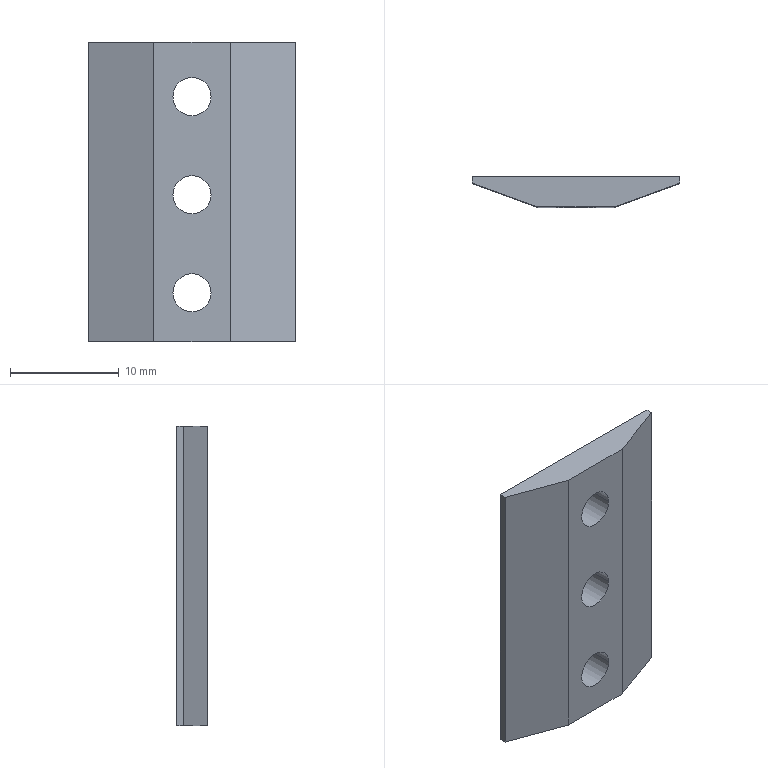Part | NX | 1 solid | 14 faces | box 19 x 2.8 x 27.5 mm | volume 1022 mm3 | plane 8 | cylinder 6 | commonest cylinder face diameters 3.5 x6
STEP:
#1=CARTESIAN_POINT('',(19.,2.8,0.));
#2=VERTEX_POINT('',#1);
#3=CARTESIAN_POINT('',(0.,2.8,0.));
#4=VERTEX_POINT('',#3);
#5=CARTESIAN_POINT('',(0.,2.8,0.));
#6=DIRECTION('',(-1.,0.,0.));
#7=VECTOR('',#6,1000.);
#8=LINE('',#5,#7);
#9=EDGE_CURVE('',#2,#4,#8,.T.);
#10=ORIENTED_EDGE('',*,*,#9,.F.);
#11=CARTESIAN_POINT('',(19.,2.8,-27.5));
#12=VERTEX_POINT('',#11);
#13=CARTESIAN_POINT('',(19.,2.8,0.));
#14=DIRECTION('',(0.,0.,1.));
#15=VECTOR('',#14,1000.);
#16=LINE('',#13,#15);
#17=EDGE_CURVE('',#12,#2,#16,.T.);
#18=ORIENTED_EDGE('',*,*,#17,.F.);
#19=CARTESIAN_POINT('',(0.,2.8,-27.5));
#20=VERTEX_POINT('',#19);
#21=CARTESIAN_POINT('',(0.,2.8,-27.5));
#22=DIRECTION('',(1.,0.,0.));
#23=VECTOR('',#22,1000.);
#24=LINE('',#21,#23);
#25=EDGE_CURVE('',#20,#12,#24,.T.);
#26=ORIENTED_EDGE('',*,*,#25,.F.);
#27=CARTESIAN_POINT('',(0.,2.8,0.));
#28=DIRECTION('',(0.,0.,-1.));
#29=VECTOR('',#28,1000.);
#30=LINE('',#27,#29);
#31=EDGE_CURVE('',#4,#20,#30,.T.);
#32=ORIENTED_EDGE('',*,*,#31,.F.);
#33=EDGE_LOOP('',(#10,#18,#26,#32));
#34=FACE_BOUND('',#33,.T.);
#35=CARTESIAN_POINT('',(11.25,2.8,-23.));
#36=VERTEX_POINT('',#35);
#37=CARTESIAN_POINT('',(7.75,2.8,-23.));
#38=VERTEX_POINT('',#37);
#39=CARTESIAN_POINT('',(9.5,2.8,-23.));
#40=DIRECTION('',(0.,-1.,0.));
#41=DIRECTION('',(1.,0.,0.));
#42=AXIS2_PLACEMENT_3D('',#39,#40,#41);
#43=CIRCLE('',#42,1.75);
#44=EDGE_CURVE('',#36,#38,#43,.T.);
#45=ORIENTED_EDGE('',*,*,#44,.T.);
#46=CARTESIAN_POINT('',(9.5,2.8,-23.));
#47=DIRECTION('',(0.,-1.,0.));
#48=DIRECTION('',(1.,0.,0.));
#49=AXIS2_PLACEMENT_3D('',#46,#47,#48);
#50=CIRCLE('',#49,1.75);
#51=EDGE_CURVE('',#38,#36,#50,.T.);
#52=ORIENTED_EDGE('',*,*,#51,.T.);
#53=EDGE_LOOP('',(#45,#52));
#54=FACE_BOUND('',#53,.T.);
#55=CARTESIAN_POINT('',(11.25,2.8,-5.));
#56=VERTEX_POINT('',#55);
#57=CARTESIAN_POINT('',(7.75,2.8,-5.));
#58=VERTEX_POINT('',#57);
#59=CARTESIAN_POINT('',(9.5,2.8,-5.));
#60=DIRECTION('',(0.,-1.,0.));
#61=DIRECTION('',(1.,0.,0.));
#62=AXIS2_PLACEMENT_3D('',#59,#60,#61);
#63=CIRCLE('',#62,1.75);
#64=EDGE_CURVE('',#56,#58,#63,.T.);
#65=ORIENTED_EDGE('',*,*,#64,.T.);
#66=CARTESIAN_POINT('',(9.5,2.8,-5.));
#67=DIRECTION('',(0.,-1.,0.));
#68=DIRECTION('',(1.,0.,0.));
#69=AXIS2_PLACEMENT_3D('',#66,#67,#68);
#70=CIRCLE('',#69,1.75);
#71=EDGE_CURVE('',#58,#56,#70,.T.);
#72=ORIENTED_EDGE('',*,*,#71,.T.);
#73=EDGE_LOOP('',(#65,#72));
#74=FACE_BOUND('',#73,.T.);
#75=CARTESIAN_POINT('',(7.75,2.8,-14.));
#76=VERTEX_POINT('',#75);
#77=CARTESIAN_POINT('',(11.25,2.8,-14.));
#78=VERTEX_POINT('',#77);
#79=CARTESIAN_POINT('',(9.5,2.8,-14.));
#80=DIRECTION('',(0.,-1.,0.));
#81=DIRECTION('',(1.,0.,0.));
#82=AXIS2_PLACEMENT_3D('',#79,#80,#81);
#83=CIRCLE('',#82,1.75);
#84=EDGE_CURVE('',#76,#78,#83,.T.);
#85=ORIENTED_EDGE('',*,*,#84,.T.);
#86=CARTESIAN_POINT('',(9.5,2.8,-14.));
#87=DIRECTION('',(0.,-1.,0.));
#88=DIRECTION('',(1.,0.,0.));
#89=AXIS2_PLACEMENT_3D('',#86,#87,#88);
#90=CIRCLE('',#89,1.75);
#91=EDGE_CURVE('',#78,#76,#90,.T.);
#92=ORIENTED_EDGE('',*,*,#91,.T.);
#93=EDGE_LOOP('',(#85,#92));
#94=FACE_BOUND('',#93,.T.);
#95=CARTESIAN_POINT('',(0.,2.8,0.));
#96=DIRECTION('',(0.,1.,0.));
#97=DIRECTION('',(1.,0.,0.));
#98=AXIS2_PLACEMENT_3D('',#95,#96,#97);
#99=PLANE('',#98);
#100=ADVANCED_FACE('',(#34,#54,#74,#94),#99,.T.);
#101=CARTESIAN_POINT('',(13.,0.,0.));
#102=VERTEX_POINT('',#101);
#103=CARTESIAN_POINT('',(6.,0.,0.));
#104=VERTEX_POINT('',#103);
#105=CARTESIAN_POINT('',(0.,0.,0.));
#106=DIRECTION('',(-1.,0.,0.));
#107=VECTOR('',#106,1000.);
#108=LINE('',#105,#107);
#109=EDGE_CURVE('',#102,#104,#108,.T.);
#110=ORIENTED_EDGE('',*,*,#109,.F.);
#111=CARTESIAN_POINT('',(19.,2.184,0.));
#112=VERTEX_POINT('',#111);
#113=CARTESIAN_POINT('',(0.,-4.732,0.));
#114=DIRECTION('',(0.9397,0.342,0.));
#115=VECTOR('',#114,1000.);
#116=LINE('',#113,#115);
#117=EDGE_CURVE('',#102,#112,#116,.T.);
#118=ORIENTED_EDGE('',*,*,#117,.T.);
#119=CARTESIAN_POINT('',(19.,0.,0.));
#120=DIRECTION('',(0.,1.,0.));
#121=VECTOR('',#120,1000.);
#122=LINE('',#119,#121);
#123=EDGE_CURVE('',#112,#2,#122,.T.);
#124=ORIENTED_EDGE('',*,*,#123,.T.);
#125=ORIENTED_EDGE('',*,*,#9,.T.);
#126=CARTESIAN_POINT('',(0.,2.184,0.));
#127=VERTEX_POINT('',#126);
#128=CARTESIAN_POINT('',(0.,0.,0.));
#129=DIRECTION('',(0.,-1.,0.));
#130=VECTOR('',#129,1000.);
#131=LINE('',#128,#130);
#132=EDGE_CURVE('',#4,#127,#131,.T.);
#133=ORIENTED_EDGE('',*,*,#132,.T.);
#134=CARTESIAN_POINT('',(0.,2.184,0.));
#135=DIRECTION('',(0.9397,-0.342,0.));
#136=VECTOR('',#135,1000.);
#137=LINE('',#134,#136);
#138=EDGE_CURVE('',#127,#104,#137,.T.);
#139=ORIENTED_EDGE('',*,*,#138,.T.);
#140=EDGE_LOOP('',(#110,#118,#124,#125,#133,#139));
#141=FACE_BOUND('',#140,.T.);
#142=CARTESIAN_POINT('',(0.,0.,0.));
#143=DIRECTION('',(0.,0.,1.));
#144=DIRECTION('',(1.,0.,0.));
#145=AXIS2_PLACEMENT_3D('',#142,#143,#144);
#146=PLANE('',#145);
#147=ADVANCED_FACE('',(#141),#146,.T.);
#148=CARTESIAN_POINT('',(6.,0.,-27.5));
#149=VERTEX_POINT('',#148);
#150=CARTESIAN_POINT('',(6.,0.,0.));
#151=DIRECTION('',(0.,0.,-1.));
#152=VECTOR('',#151,1000.);
#153=LINE('',#150,#152);
#154=EDGE_CURVE('',#104,#149,#153,.T.);
#155=ORIENTED_EDGE('',*,*,#154,.F.);
#156=ORIENTED_EDGE('',*,*,#138,.F.);
#157=CARTESIAN_POINT('',(0.,2.184,-27.5));
#158=VERTEX_POINT('',#157);
#159=CARTESIAN_POINT('',(0.,2.184,0.));
#160=DIRECTION('',(0.,0.,1.));
#161=VECTOR('',#160,1000.);
#162=LINE('',#159,#161);
#163=EDGE_CURVE('',#158,#127,#162,.T.);
#164=ORIENTED_EDGE('',*,*,#163,.F.);
#165=CARTESIAN_POINT('',(0.,2.184,-27.5));
#166=DIRECTION('',(0.9397,-0.342,0.));
#167=VECTOR('',#166,1000.);
#168=LINE('',#165,#167);
#169=EDGE_CURVE('',#158,#149,#168,.T.);
#170=ORIENTED_EDGE('',*,*,#169,.T.);
#171=EDGE_LOOP('',(#155,#156,#164,#170));
#172=FACE_BOUND('',#171,.T.);
#173=CARTESIAN_POINT('',(6.,0.,-28.));
#174=DIRECTION('',(-0.342,-0.9397,0.));
#175=DIRECTION('',(-0.9397,0.342,0.));
#176=AXIS2_PLACEMENT_3D('',#173,#174,#175);
#177=PLANE('',#176);
#178=ADVANCED_FACE('',(#172),#177,.T.);
#179=CARTESIAN_POINT('',(13.,0.,-27.5));
#180=VERTEX_POINT('',#179);
#181=CARTESIAN_POINT('',(0.,0.,-27.5));
#182=DIRECTION('',(-1.,0.,0.));
#183=VECTOR('',#182,1000.);
#184=LINE('',#181,#183);
#185=EDGE_CURVE('',#180,#149,#184,.T.);
#186=ORIENTED_EDGE('',*,*,#185,.T.);
#187=ORIENTED_EDGE('',*,*,#169,.F.);
#188=CARTESIAN_POINT('',(0.,0.,-27.5));
#189=DIRECTION('',(0.,-1.,0.));
#190=VECTOR('',#189,1000.);
#191=LINE('',#188,#190);
#192=EDGE_CURVE('',#20,#158,#191,.T.);
#193=ORIENTED_EDGE('',*,*,#192,.F.);
#194=ORIENTED_EDGE('',*,*,#25,.T.);
#195=CARTESIAN_POINT('',(19.,2.184,-27.5));
#196=VERTEX_POINT('',#195);
#197=CARTESIAN_POINT('',(19.,0.,-27.5));
#198=DIRECTION('',(0.,1.,0.));
#199=VECTOR('',#198,1000.);
#200=LINE('',#197,#199);
#201=EDGE_CURVE('',#196,#12,#200,.T.);
#202=ORIENTED_EDGE('',*,*,#201,.F.);
#203=CARTESIAN_POINT('',(0.,-4.732,-27.5));
#204=DIRECTION('',(0.9397,0.342,0.));
#205=VECTOR('',#204,1000.);
#206=LINE('',#203,#205);
#207=EDGE_CURVE('',#180,#196,#206,.T.);
#208=ORIENTED_EDGE('',*,*,#207,.F.);
#209=EDGE_LOOP('',(#186,#187,#193,#194,#202,#208));
#210=FACE_BOUND('',#209,.T.);
#211=CARTESIAN_POINT('',(19.,0.,-27.5));
#212=DIRECTION('',(0.,0.,-1.));
#213=DIRECTION('',(0.,-1.,0.));
#214=AXIS2_PLACEMENT_3D('',#211,#212,#213);
#215=PLANE('',#214);
#216=ADVANCED_FACE('',(#210),#215,.T.);
#217=CARTESIAN_POINT('',(13.,0.,0.));
#218=DIRECTION('',(0.,0.,1.));
#219=VECTOR('',#218,1000.);
#220=LINE('',#217,#219);
#221=EDGE_CURVE('',#180,#102,#220,.T.);
#222=ORIENTED_EDGE('',*,*,#221,.F.);
#223=ORIENTED_EDGE('',*,*,#207,.T.);
#224=CARTESIAN_POINT('',(19.,2.184,0.));
#225=DIRECTION('',(0.,0.,-1.));
#226=VECTOR('',#225,1000.);
#227=LINE('',#224,#226);
#228=EDGE_CURVE('',#112,#196,#227,.T.);
#229=ORIENTED_EDGE('',*,*,#228,.F.);
#230=ORIENTED_EDGE('',*,*,#117,.F.);
#231=EDGE_LOOP('',(#222,#223,#229,#230));
#232=FACE_BOUND('',#231,.T.);
#233=CARTESIAN_POINT('',(13.,0.,0.));
#234=DIRECTION('',(0.342,-0.9397,0.));
#235=DIRECTION('',(0.,0.,-1.));
#236=AXIS2_PLACEMENT_3D('',#233,#234,#235);
#237=PLANE('',#236);
#238=ADVANCED_FACE('',(#232),#237,.T.);
#239=ORIENTED_EDGE('',*,*,#228,.T.);
#240=ORIENTED_EDGE('',*,*,#201,.T.);
#241=ORIENTED_EDGE('',*,*,#17,.T.);
#242=ORIENTED_EDGE('',*,*,#123,.F.);
#243=EDGE_LOOP('',(#239,#240,#241,#242));
#244=FACE_BOUND('',#243,.T.);
#245=CARTESIAN_POINT('',(19.,0.,0.));
#246=DIRECTION('',(1.,0.,0.));
#247=DIRECTION('',(0.,1.,0.));
#248=AXIS2_PLACEMENT_3D('',#245,#246,#247);
#249=PLANE('',#248);
#250=ADVANCED_FACE('',(#244),#249,.T.);
#251=ORIENTED_EDGE('',*,*,#109,.T.);
#252=ORIENTED_EDGE('',*,*,#154,.T.);
#253=ORIENTED_EDGE('',*,*,#185,.F.);
#254=ORIENTED_EDGE('',*,*,#221,.T.);
#255=EDGE_LOOP('',(#251,#252,#253,#254));
#256=FACE_BOUND('',#255,.T.);
#257=CARTESIAN_POINT('',(11.25,0.,-23.));
#258=VERTEX_POINT('',#257);
#259=CARTESIAN_POINT('',(7.75,0.,-23.));
#260=VERTEX_POINT('',#259);
#261=CARTESIAN_POINT('',(9.5,0.,-23.));
#262=DIRECTION('',(0.,-1.,0.));
#263=DIRECTION('',(1.,0.,0.));
#264=AXIS2_PLACEMENT_3D('',#261,#262,#263);
#265=CIRCLE('',#264,1.75);
#266=EDGE_CURVE('',#258,#260,#265,.T.);
#267=ORIENTED_EDGE('',*,*,#266,.F.);
#268=CARTESIAN_POINT('',(9.5,0.,-23.));
#269=DIRECTION('',(0.,-1.,0.));
#270=DIRECTION('',(1.,0.,0.));
#271=AXIS2_PLACEMENT_3D('',#268,#269,#270);
#272=CIRCLE('',#271,1.75);
#273=EDGE_CURVE('',#260,#258,#272,.T.);
#274=ORIENTED_EDGE('',*,*,#273,.F.);
#275=EDGE_LOOP('',(#267,#274));
#276=FACE_BOUND('',#275,.T.);
#277=CARTESIAN_POINT('',(11.25,0.,-5.));
#278=VERTEX_POINT('',#277);
#279=CARTESIAN_POINT('',(7.75,0.,-5.));
#280=VERTEX_POINT('',#279);
#281=CARTESIAN_POINT('',(9.5,0.,-5.));
#282=DIRECTION('',(0.,-1.,0.));
#283=DIRECTION('',(1.,0.,0.));
#284=AXIS2_PLACEMENT_3D('',#281,#282,#283);
#285=CIRCLE('',#284,1.75);
#286=EDGE_CURVE('',#278,#280,#285,.T.);
#287=ORIENTED_EDGE('',*,*,#286,.F.);
#288=CARTESIAN_POINT('',(9.5,0.,-5.));
#289=DIRECTION('',(0.,-1.,0.));
#290=DIRECTION('',(1.,0.,0.));
#291=AXIS2_PLACEMENT_3D('',#288,#289,#290);
#292=CIRCLE('',#291,1.75);
#293=EDGE_CURVE('',#280,#278,#292,.T.);
#294=ORIENTED_EDGE('',*,*,#293,.F.);
#295=EDGE_LOOP('',(#287,#294));
#296=FACE_BOUND('',#295,.T.);
#297=CARTESIAN_POINT('',(11.25,0.,-14.));
#298=VERTEX_POINT('',#297);
#299=CARTESIAN_POINT('',(7.75,0.,-14.));
#300=VERTEX_POINT('',#299);
#301=CARTESIAN_POINT('',(9.5,0.,-14.));
#302=DIRECTION('',(0.,-1.,0.));
#303=DIRECTION('',(1.,0.,0.));
#304=AXIS2_PLACEMENT_3D('',#301,#302,#303);
#305=CIRCLE('',#304,1.75);
#306=EDGE_CURVE('',#298,#300,#305,.T.);
#307=ORIENTED_EDGE('',*,*,#306,.F.);
#308=CARTESIAN_POINT('',(9.5,0.,-14.));
#309=DIRECTION('',(0.,-1.,0.));
#310=DIRECTION('',(1.,0.,0.));
#311=AXIS2_PLACEMENT_3D('',#308,#309,#310);
#312=CIRCLE('',#311,1.75);
#313=EDGE_CURVE('',#300,#298,#312,.T.);
#314=ORIENTED_EDGE('',*,*,#313,.F.);
#315=EDGE_LOOP('',(#307,#314));
#316=FACE_BOUND('',#315,.T.);
#317=CARTESIAN_POINT('',(0.,0.,0.));
#318=DIRECTION('',(0.,1.,0.));
#319=DIRECTION('',(1.,0.,0.));
#320=AXIS2_PLACEMENT_3D('',#317,#318,#319);
#321=PLANE('',#320);
#322=ADVANCED_FACE('',(#256,#276,#296,#316),#321,.F.);
#323=ORIENTED_EDGE('',*,*,#163,.T.);
#324=ORIENTED_EDGE('',*,*,#132,.F.);
#325=ORIENTED_EDGE('',*,*,#31,.T.);
#326=ORIENTED_EDGE('',*,*,#192,.T.);
#327=EDGE_LOOP('',(#323,#324,#325,#326));
#328=FACE_BOUND('',#327,.T.);
#329=CARTESIAN_POINT('',(0.,0.,-28.));
#330=DIRECTION('',(-1.,0.,0.));
#331=DIRECTION('',(0.,0.,1.));
#332=AXIS2_PLACEMENT_3D('',#329,#330,#331);
#333=PLANE('',#332);
#334=ADVANCED_FACE('',(#328),#333,.T.);
#335=ORIENTED_EDGE('',*,*,#266,.T.);
#336=CARTESIAN_POINT('',(7.75,2.8,-23.));
#337=DIRECTION('',(0.,-1.,0.));
#338=VECTOR('',#337,1000.);
#339=LINE('',#336,#338);
#340=EDGE_CURVE('',#38,#260,#339,.T.);
#341=ORIENTED_EDGE('',*,*,#340,.F.);
#342=ORIENTED_EDGE('',*,*,#44,.F.);
#343=CARTESIAN_POINT('',(11.25,2.8,-23.));
#344=DIRECTION('',(0.,-1.,0.));
#345=VECTOR('',#344,1000.);
#346=LINE('',#343,#345);
#347=EDGE_CURVE('',#36,#258,#346,.T.);
#348=ORIENTED_EDGE('',*,*,#347,.T.);
#349=EDGE_LOOP('',(#335,#341,#342,#348));
#350=FACE_BOUND('',#349,.T.);
#351=CARTESIAN_POINT('',(9.5,2.8,-23.));
#352=DIRECTION('',(0.,-1.,0.));
#353=DIRECTION('',(1.,0.,0.));
#354=AXIS2_PLACEMENT_3D('',#351,#352,#353);
#355=CYLINDRICAL_SURFACE('',#354,1.75);
#356=ADVANCED_FACE('',(#350),#355,.F.);
#357=ORIENTED_EDGE('',*,*,#306,.T.);
#358=CARTESIAN_POINT('',(7.75,2.8,-14.));
#359=DIRECTION('',(0.,-1.,0.));
#360=VECTOR('',#359,1000.);
#361=LINE('',#358,#360);
#362=EDGE_CURVE('',#300,#76,#361,.F.);
#363=ORIENTED_EDGE('',*,*,#362,.T.);
#364=ORIENTED_EDGE('',*,*,#91,.F.);
#365=CARTESIAN_POINT('',(11.25,2.8,-14.));
#366=DIRECTION('',(0.,-1.,0.));
#367=VECTOR('',#366,1000.);
#368=LINE('',#365,#367);
#369=EDGE_CURVE('',#298,#78,#368,.F.);
#370=ORIENTED_EDGE('',*,*,#369,.F.);
#371=EDGE_LOOP('',(#357,#363,#364,#370));
#372=FACE_BOUND('',#371,.T.);
#373=CARTESIAN_POINT('',(9.5,2.8,-14.));
#374=DIRECTION('',(0.,-1.,0.));
#375=DIRECTION('',(1.,0.,0.));
#376=AXIS2_PLACEMENT_3D('',#373,#374,#375);
#377=CYLINDRICAL_SURFACE('',#376,1.75);
#378=ADVANCED_FACE('',(#372),#377,.F.);
#379=ORIENTED_EDGE('',*,*,#64,.F.);
#380=CARTESIAN_POINT('',(11.25,2.8,-5.));
#381=DIRECTION('',(0.,-1.,0.));
#382=VECTOR('',#381,1000.);
#383=LINE('',#380,#382);
#384=EDGE_CURVE('',#56,#278,#383,.T.);
#385=ORIENTED_EDGE('',*,*,#384,.T.);
#386=ORIENTED_EDGE('',*,*,#286,.T.);
#387=CARTESIAN_POINT('',(7.75,2.8,-5.));
#388=DIRECTION('',(0.,-1.,0.));
#389=VECTOR('',#388,1000.);
#390=LINE('',#387,#389);
#391=EDGE_CURVE('',#58,#280,#390,.T.);
#392=ORIENTED_EDGE('',*,*,#391,.F.);
#393=EDGE_LOOP('',(#379,#385,#386,#392));
#394=FACE_BOUND('',#393,.T.);
#395=CARTESIAN_POINT('',(9.5,2.8,-5.));
#396=DIRECTION('',(0.,-1.,0.));
#397=DIRECTION('',(1.,0.,0.));
#398=AXIS2_PLACEMENT_3D('',#395,#396,#397);
#399=CYLINDRICAL_SURFACE('',#398,1.75);
#400=ADVANCED_FACE('',(#394),#399,.F.);
#401=ORIENTED_EDGE('',*,*,#347,.F.);
#402=ORIENTED_EDGE('',*,*,#51,.F.);
#403=ORIENTED_EDGE('',*,*,#340,.T.);
#404=ORIENTED_EDGE('',*,*,#273,.T.);
#405=EDGE_LOOP('',(#401,#402,#403,#404));
#406=FACE_BOUND('',#405,.T.);
#407=CARTESIAN_POINT('',(9.5,2.8,-23.));
#408=DIRECTION('',(0.,-1.,0.));
#409=DIRECTION('',(1.,0.,0.));
#410=AXIS2_PLACEMENT_3D('',#407,#408,#409);
#411=CYLINDRICAL_SURFACE('',#410,1.75);
#412=ADVANCED_FACE('',(#406),#411,.F.);
#413=ORIENTED_EDGE('',*,*,#84,.F.);
#414=ORIENTED_EDGE('',*,*,#362,.F.);
#415=ORIENTED_EDGE('',*,*,#313,.T.);
#416=ORIENTED_EDGE('',*,*,#369,.T.);
#417=EDGE_LOOP('',(#413,#414,#415,#416));
#418=FACE_BOUND('',#417,.T.);
#419=CARTESIAN_POINT('',(9.5,2.8,-14.));
#420=DIRECTION('',(0.,-1.,0.));
#421=DIRECTION('',(1.,0.,0.));
#422=AXIS2_PLACEMENT_3D('',#419,#420,#421);
#423=CYLINDRICAL_SURFACE('',#422,1.75);
#424=ADVANCED_FACE('',(#418),#423,.F.);
#425=ORIENTED_EDGE('',*,*,#384,.F.);
#426=ORIENTED_EDGE('',*,*,#71,.F.);
#427=ORIENTED_EDGE('',*,*,#391,.T.);
#428=ORIENTED_EDGE('',*,*,#293,.T.);
#429=EDGE_LOOP('',(#425,#426,#427,#428));
#430=FACE_BOUND('',#429,.T.);
#431=CARTESIAN_POINT('',(9.5,2.8,-5.));
#432=DIRECTION('',(0.,-1.,0.));
#433=DIRECTION('',(1.,0.,0.));
#434=AXIS2_PLACEMENT_3D('',#431,#432,#433);
#435=CYLINDRICAL_SURFACE('',#434,1.75);
#436=ADVANCED_FACE('',(#430),#435,.F.);
#437=CLOSED_SHELL('',(#100,#147,#178,#216,#238,#250,#322,#334,#356,#378,#400,#412,#424,#436));
#438=MANIFOLD_SOLID_BREP('',#437);
#439=(LENGTH_UNIT()NAMED_UNIT(*)SI_UNIT(.MILLI.,.METRE.));
#440=UNCERTAINTY_MEASURE_WITH_UNIT(LENGTH_MEASURE(0.00001),#439,'','');
#441=(NAMED_UNIT(*)PLANE_ANGLE_UNIT()SI_UNIT($,.RADIAN.));
#442=(NAMED_UNIT(*)SI_UNIT($,.STERADIAN.)SOLID_ANGLE_UNIT());
#443=(GEOMETRIC_REPRESENTATION_CONTEXT(3)GLOBAL_UNCERTAINTY_ASSIGNED_CONTEXT((#440))GLOBAL_UNIT_ASSIGNED_CONTEXT((#439,#441,#442))REPRESENTATION_CONTEXT('',''));
#444=ADVANCED_BREP_SHAPE_REPRESENTATION('',(#438),#443);